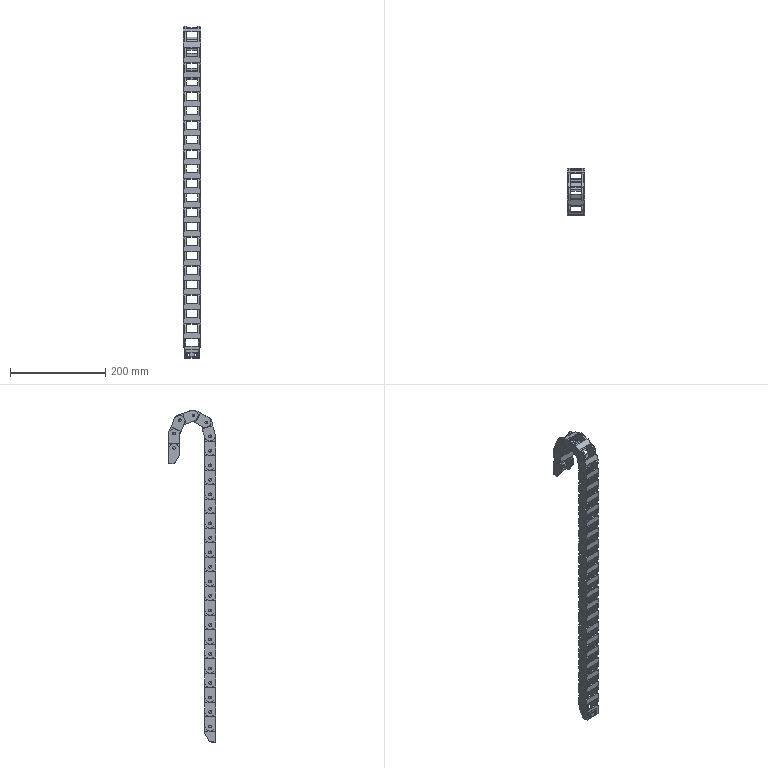Part | SolidWorks | 27 solids | 1687 faces | box 36.5 x 99.183 x 698.245 mm | volume 224185 mm3 | plane 874 | cylinder 801 | cone 8 | torus 4 | commonest cylinder face diameters 1 x270 6 x204 5.9 x100 16.02 x50 18.716 x50 19.5 x50